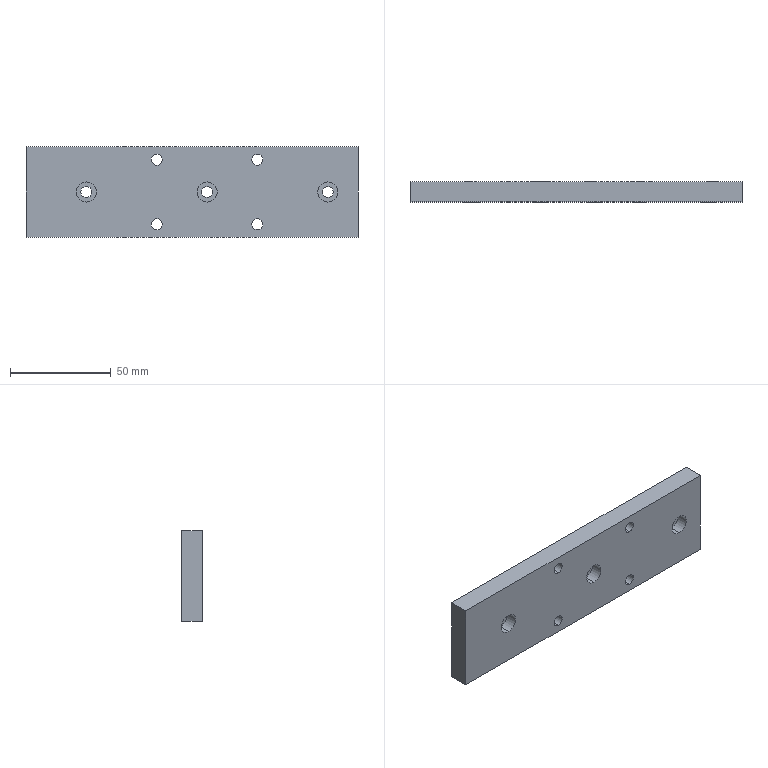Part | STEP file | Grinding bracket base plate | 1 solid | 41 faces | box 165 x 10 x 45 mm | volume 70401 mm3 | cylinder 28 | plane 13 | commonest cylinder face diameters 5.5 x14 10 x14